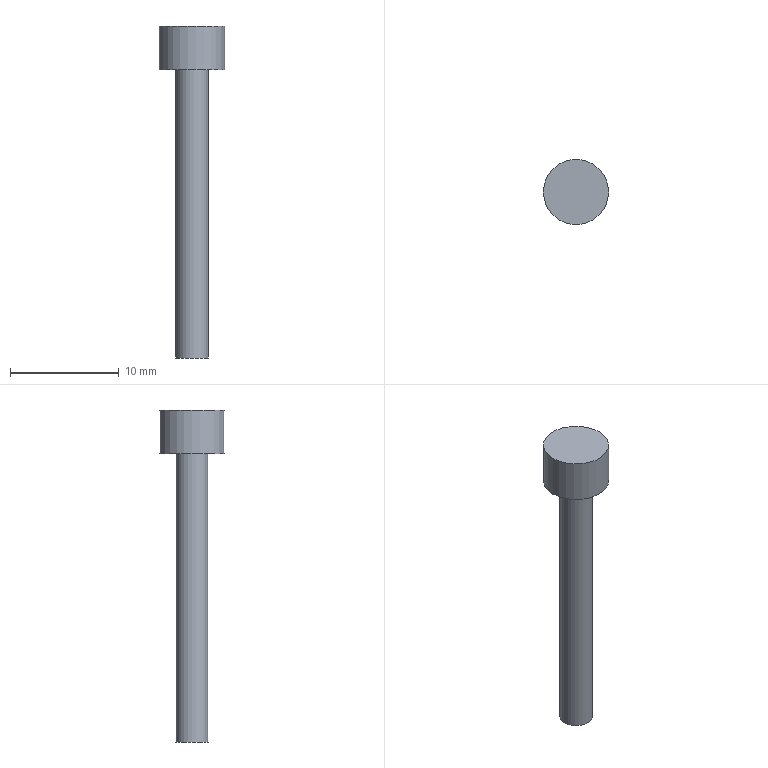Part | STEP file | 1 solid | 5 faces | box 6 x 6 x 30.5 mm | volume 300.415 mm3 | plane 3 | cylinder 2 | commonest cylinder face diameters 3 x1 6 x1
STEP:
#1=CARTESIAN_POINT('',(0.,0.,0.));
#2=DIRECTION('',(0.,0.,1.));
#3=DIRECTION('',(1.,0.,0.));
#4=AXIS2_PLACEMENT_3D('',#1,#2,#3);
#5=CARTESIAN_POINT('',(1371.362,477.495,17.579));
#6=VERTEX_POINT('',#5);
#7=CARTESIAN_POINT('',(1372.862,477.495,17.579));
#8=DIRECTION('',(0.,0.,1.));
#9=DIRECTION('',(-1.,0.,0.));
#10=AXIS2_PLACEMENT_3D('',#7,#8,#9);
#11=CIRCLE('',#10,1.5);
#12=CARTESIAN_POINT('',(1372.862,477.495,17.579));
#13=DIRECTION('',(0.,0.,-1.));
#14=DIRECTION('',(-1.,0.,0.));
#15=AXIS2_PLACEMENT_3D('',#12,#13,#14);
#16=PLANE('',#15);
#17=CARTESIAN_POINT('',(1.5,0.));
#18=CARTESIAN_POINT('',(1.5,-2.598));
#19=CARTESIAN_POINT('',(-0.75,-1.299));
#20=CARTESIAN_POINT('',(-3.,0.));
#21=CARTESIAN_POINT('',(-0.75,1.299));
#22=CARTESIAN_POINT('',(1.5,2.598));
#23=CARTESIAN_POINT('',(1.5,0.));
#24=(BOUNDED_CURVE()B_SPLINE_CURVE(2,(#17,#18,#19,#20,#21,#22,#23),.UNSPECIFIED.,.T.,.F.)B_SPLINE_CURVE_WITH_KNOTS((1,2,2,2,2,1),(-2.094,0.,2.094,4.189,6.283,8.378),.UNSPECIFIED.)CURVE()GEOMETRIC_REPRESENTATION_ITEM()RATIONAL_B_SPLINE_CURVE((1.,0.5,1.,0.5,1.,0.5,1.))REPRESENTATION_ITEM(''));
#25=(GEOMETRIC_REPRESENTATION_CONTEXT(2)PARAMETRIC_REPRESENTATION_CONTEXT()REPRESENTATION_CONTEXT('',''));
#26=DEFINITIONAL_REPRESENTATION('',(#24),#25);
#27=PCURVE('',#16,#26);
#28=CARTESIAN_POINT('',(1372.862,477.495,43.879));
#29=DIRECTION('',(0.,0.,-1.));
#30=DIRECTION('',(-1.,0.,0.));
#31=AXIS2_PLACEMENT_3D('',#28,#29,#30);
#32=CYLINDRICAL_SURFACE('',#31,1.5);
#33=CARTESIAN_POINT('',(6.283,26.3));
#34=DIRECTION('',(-1.,0.));
#35=VECTOR('',#34,1.);
#36=LINE('',#33,#35);
#37=(GEOMETRIC_REPRESENTATION_CONTEXT(2)PARAMETRIC_REPRESENTATION_CONTEXT()REPRESENTATION_CONTEXT('',''));
#38=DEFINITIONAL_REPRESENTATION('',(#36),#37);
#39=PCURVE('',#32,#38);
#40=SURFACE_CURVE('',#11,(#27,#39),.PCURVE_S1.);
#41=EDGE_CURVE('',#6,#6,#40,.T.);
#42=ORIENTED_EDGE('',*,*,#41,.F.);
#43=EDGE_LOOP('',(#42));
#44=FACE_BOUND('',#43,.T.);
#45=ADVANCED_FACE('',(#44),#16,.T.);
#46=ORIENTED_EDGE('',*,*,#41,.T.);
#47=CARTESIAN_POINT('',(1371.362,477.495,44.079));
#48=VERTEX_POINT('',#47);
#49=CARTESIAN_POINT('',(1371.362,477.495,44.079));
#50=CARTESIAN_POINT('',(1371.362,477.495,17.579));
#51=B_SPLINE_CURVE_WITH_KNOTS('',1,(#49,#50),.UNSPECIFIED.,.F.,.F.,(2,2),(-0.2,26.3),.PIECEWISE_BEZIER_KNOTS.);
#52=CARTESIAN_POINT('',(0.,0.));
#53=DIRECTION('',(0.,1.));
#54=VECTOR('',#53,1.);
#55=LINE('',#52,#54);
#56=(GEOMETRIC_REPRESENTATION_CONTEXT(2)PARAMETRIC_REPRESENTATION_CONTEXT()REPRESENTATION_CONTEXT('',''));
#57=DEFINITIONAL_REPRESENTATION('',(#55),#56);
#58=PCURVE('',#32,#57);
#59=CARTESIAN_POINT('',(6.283,0.));
#60=DIRECTION('',(0.,1.));
#61=VECTOR('',#60,1.);
#62=LINE('',#59,#61);
#63=(GEOMETRIC_REPRESENTATION_CONTEXT(2)PARAMETRIC_REPRESENTATION_CONTEXT()REPRESENTATION_CONTEXT('',''));
#64=DEFINITIONAL_REPRESENTATION('',(#62),#63);
#65=PCURVE('',#32,#64);
#66=SEAM_CURVE('',#51,(#58,#65),.PCURVE_S1.);
#67=EDGE_CURVE('',#48,#6,#66,.T.);
#68=ORIENTED_EDGE('',*,*,#67,.F.);
#69=CARTESIAN_POINT('',(1374.362,477.495,44.079));
#70=VERTEX_POINT('',#69);
#71=CARTESIAN_POINT('',(1372.862,477.495,44.079));
#72=DIRECTION('',(0.,0.,1.));
#73=DIRECTION('',(1.,0.,0.));
#74=AXIS2_PLACEMENT_3D('',#71,#72,#73);
#75=CIRCLE('',#74,1.5);
#76=CARTESIAN_POINT('',(3.142,-0.2));
#77=DIRECTION('',(-1.,0.));
#78=VECTOR('',#77,1.);
#79=LINE('',#76,#78);
#80=(GEOMETRIC_REPRESENTATION_CONTEXT(2)PARAMETRIC_REPRESENTATION_CONTEXT()REPRESENTATION_CONTEXT('',''));
#81=DEFINITIONAL_REPRESENTATION('',(#79),#80);
#82=PCURVE('',#32,#81);
#83=CARTESIAN_POINT('',(1372.862,477.495,44.079));
#84=DIRECTION('',(0.,0.,-1.));
#85=DIRECTION('',(-1.,0.,0.));
#86=AXIS2_PLACEMENT_3D('',#83,#84,#85);
#87=PLANE('',#86);
#88=CARTESIAN_POINT('',(-1.5,0.));
#89=CARTESIAN_POINT('',(-1.5,2.598));
#90=CARTESIAN_POINT('',(0.75,1.299));
#91=CARTESIAN_POINT('',(3.,0.));
#92=CARTESIAN_POINT('',(0.75,-1.299));
#93=CARTESIAN_POINT('',(-1.5,-2.598));
#94=CARTESIAN_POINT('',(-1.5,0.));
#95=(BOUNDED_CURVE()B_SPLINE_CURVE(2,(#88,#89,#90,#91,#92,#93,#94),.UNSPECIFIED.,.T.,.F.)B_SPLINE_CURVE_WITH_KNOTS((1,2,2,2,2,1),(-2.094,0.,2.094,4.189,6.283,8.378),.UNSPECIFIED.)CURVE()GEOMETRIC_REPRESENTATION_ITEM()RATIONAL_B_SPLINE_CURVE((1.,0.5,1.,0.5,1.,0.5,1.))REPRESENTATION_ITEM(''));
#96=(GEOMETRIC_REPRESENTATION_CONTEXT(2)PARAMETRIC_REPRESENTATION_CONTEXT()REPRESENTATION_CONTEXT('',''));
#97=DEFINITIONAL_REPRESENTATION('',(#95),#96);
#98=PCURVE('',#87,#97);
#99=SURFACE_CURVE('',#75,(#82,#98),.PCURVE_S1.);
#100=EDGE_CURVE('',#70,#48,#99,.T.);
#101=ORIENTED_EDGE('',*,*,#100,.F.);
#102=CARTESIAN_POINT('',(1372.862,477.495,44.079));
#103=DIRECTION('',(0.,0.,1.));
#104=DIRECTION('',(1.,0.,0.));
#105=AXIS2_PLACEMENT_3D('',#102,#103,#104);
#106=CIRCLE('',#105,1.5);
#107=CARTESIAN_POINT('',(9.425,-0.2));
#108=DIRECTION('',(-1.,0.));
#109=VECTOR('',#108,1.);
#110=LINE('',#107,#109);
#111=(GEOMETRIC_REPRESENTATION_CONTEXT(2)PARAMETRIC_REPRESENTATION_CONTEXT()REPRESENTATION_CONTEXT('',''));
#112=DEFINITIONAL_REPRESENTATION('',(#110),#111);
#113=PCURVE('',#32,#112);
#114=CARTESIAN_POINT('',(-1.5,0.));
#115=CARTESIAN_POINT('',(-1.5,2.598));
#116=CARTESIAN_POINT('',(0.75,1.299));
#117=CARTESIAN_POINT('',(3.,0.));
#118=CARTESIAN_POINT('',(0.75,-1.299));
#119=CARTESIAN_POINT('',(-1.5,-2.598));
#120=CARTESIAN_POINT('',(-1.5,0.));
#121=(BOUNDED_CURVE()B_SPLINE_CURVE(2,(#114,#115,#116,#117,#118,#119,#120),.UNSPECIFIED.,.T.,.F.)B_SPLINE_CURVE_WITH_KNOTS((1,2,2,2,2,1),(-2.094,0.,2.094,4.189,6.283,8.378),.UNSPECIFIED.)CURVE()GEOMETRIC_REPRESENTATION_ITEM()RATIONAL_B_SPLINE_CURVE((1.,0.5,1.,0.5,1.,0.5,1.))REPRESENTATION_ITEM(''));
#122=(GEOMETRIC_REPRESENTATION_CONTEXT(2)PARAMETRIC_REPRESENTATION_CONTEXT()REPRESENTATION_CONTEXT('',''));
#123=DEFINITIONAL_REPRESENTATION('',(#121),#122);
#124=PCURVE('',#87,#123);
#125=SURFACE_CURVE('',#106,(#113,#124),.PCURVE_S1.);
#126=EDGE_CURVE('',#48,#70,#125,.T.);
#127=ORIENTED_EDGE('',*,*,#126,.F.);
#128=ORIENTED_EDGE('',*,*,#67,.T.);
#129=EDGE_LOOP('',(#46,#68,#101,#127,#128));
#130=FACE_BOUND('',#129,.T.);
#131=ADVANCED_FACE('',(#130),#32,.T.);
#132=CARTESIAN_POINT('',(1369.862,477.495,48.079));
#133=VERTEX_POINT('',#132);
#134=CARTESIAN_POINT('',(1372.862,477.495,48.079));
#135=DIRECTION('',(0.,0.,-1.));
#136=DIRECTION('',(-1.,0.,0.));
#137=AXIS2_PLACEMENT_3D('',#134,#135,#136);
#138=CIRCLE('',#137,3.);
#139=CARTESIAN_POINT('',(1372.862,477.495,48.079));
#140=DIRECTION('',(0.,0.,1.));
#141=DIRECTION('',(1.,0.,0.));
#142=AXIS2_PLACEMENT_3D('',#139,#140,#141);
#143=PLANE('',#142);
#144=CARTESIAN_POINT('',(-3.,0.));
#145=CARTESIAN_POINT('',(-3.,5.196));
#146=CARTESIAN_POINT('',(1.5,2.598));
#147=CARTESIAN_POINT('',(6.,0.));
#148=CARTESIAN_POINT('',(1.5,-2.598));
#149=CARTESIAN_POINT('',(-3.,-5.196));
#150=CARTESIAN_POINT('',(-3.,0.));
#151=(BOUNDED_CURVE()B_SPLINE_CURVE(2,(#144,#145,#146,#147,#148,#149,#150),.UNSPECIFIED.,.T.,.F.)B_SPLINE_CURVE_WITH_KNOTS((1,2,2,2,2,1),(-2.094,0.,2.094,4.189,6.283,8.378),.UNSPECIFIED.)CURVE()GEOMETRIC_REPRESENTATION_ITEM()RATIONAL_B_SPLINE_CURVE((1.,0.5,1.,0.5,1.,0.5,1.))REPRESENTATION_ITEM(''));
#152=(GEOMETRIC_REPRESENTATION_CONTEXT(2)PARAMETRIC_REPRESENTATION_CONTEXT()REPRESENTATION_CONTEXT('',''));
#153=DEFINITIONAL_REPRESENTATION('',(#151),#152);
#154=PCURVE('',#143,#153);
#155=CARTESIAN_POINT('',(1372.862,477.495,44.079));
#156=DIRECTION('',(0.,0.,1.));
#157=DIRECTION('',(-1.,0.,0.));
#158=AXIS2_PLACEMENT_3D('',#155,#156,#157);
#159=CYLINDRICAL_SURFACE('',#158,3.);
#160=CARTESIAN_POINT('',(6.283,4.));
#161=DIRECTION('',(-1.,0.));
#162=VECTOR('',#161,1.);
#163=LINE('',#160,#162);
#164=(GEOMETRIC_REPRESENTATION_CONTEXT(2)PARAMETRIC_REPRESENTATION_CONTEXT()REPRESENTATION_CONTEXT('',''));
#165=DEFINITIONAL_REPRESENTATION('',(#163),#164);
#166=PCURVE('',#159,#165);
#167=SURFACE_CURVE('',#138,(#154,#166),.PCURVE_S1.);
#168=EDGE_CURVE('',#133,#133,#167,.T.);
#169=ORIENTED_EDGE('',*,*,#168,.F.);
#170=EDGE_LOOP('',(#169));
#171=FACE_BOUND('',#170,.T.);
#172=ADVANCED_FACE('',(#171),#143,.T.);
#173=ORIENTED_EDGE('',*,*,#100,.T.);
#174=ORIENTED_EDGE('',*,*,#126,.T.);
#175=EDGE_LOOP('',(#173,#174));
#176=FACE_BOUND('',#175,.T.);
#177=CARTESIAN_POINT('',(1375.862,477.495,44.079));
#178=VERTEX_POINT('',#177);
#179=CARTESIAN_POINT('',(1369.862,477.495,44.079));
#180=VERTEX_POINT('',#179);
#181=CARTESIAN_POINT('',(1372.862,477.495,44.079));
#182=DIRECTION('',(0.,0.,1.));
#183=DIRECTION('',(1.,0.,0.));
#184=AXIS2_PLACEMENT_3D('',#181,#182,#183);
#185=CIRCLE('',#184,3.);
#186=CARTESIAN_POINT('',(-3.,0.));
#187=CARTESIAN_POINT('',(-3.,5.196));
#188=CARTESIAN_POINT('',(1.5,2.598));
#189=CARTESIAN_POINT('',(6.,0.));
#190=CARTESIAN_POINT('',(1.5,-2.598));
#191=CARTESIAN_POINT('',(-3.,-5.196));
#192=CARTESIAN_POINT('',(-3.,0.));
#193=(BOUNDED_CURVE()B_SPLINE_CURVE(2,(#186,#187,#188,#189,#190,#191,#192),.UNSPECIFIED.,.T.,.F.)B_SPLINE_CURVE_WITH_KNOTS((1,2,2,2,2,1),(-2.094,0.,2.094,4.189,6.283,8.378),.UNSPECIFIED.)CURVE()GEOMETRIC_REPRESENTATION_ITEM()RATIONAL_B_SPLINE_CURVE((1.,0.5,1.,0.5,1.,0.5,1.))REPRESENTATION_ITEM(''));
#194=(GEOMETRIC_REPRESENTATION_CONTEXT(2)PARAMETRIC_REPRESENTATION_CONTEXT()REPRESENTATION_CONTEXT('',''));
#195=DEFINITIONAL_REPRESENTATION('',(#193),#194);
#196=PCURVE('',#87,#195);
#197=CARTESIAN_POINT('',(3.142,0.));
#198=DIRECTION('',(1.,0.));
#199=VECTOR('',#198,1.);
#200=LINE('',#197,#199);
#201=(GEOMETRIC_REPRESENTATION_CONTEXT(2)PARAMETRIC_REPRESENTATION_CONTEXT()REPRESENTATION_CONTEXT('',''));
#202=DEFINITIONAL_REPRESENTATION('',(#200),#201);
#203=PCURVE('',#159,#202);
#204=SURFACE_CURVE('',#185,(#196,#203),.PCURVE_S1.);
#205=EDGE_CURVE('',#178,#180,#204,.T.);
#206=ORIENTED_EDGE('',*,*,#205,.F.);
#207=CARTESIAN_POINT('',(1372.862,477.495,44.079));
#208=DIRECTION('',(0.,0.,1.));
#209=DIRECTION('',(1.,0.,0.));
#210=AXIS2_PLACEMENT_3D('',#207,#208,#209);
#211=CIRCLE('',#210,3.);
#212=CARTESIAN_POINT('',(-3.,0.));
#213=CARTESIAN_POINT('',(-3.,5.196));
#214=CARTESIAN_POINT('',(1.5,2.598));
#215=CARTESIAN_POINT('',(6.,0.));
#216=CARTESIAN_POINT('',(1.5,-2.598));
#217=CARTESIAN_POINT('',(-3.,-5.196));
#218=CARTESIAN_POINT('',(-3.,0.));
#219=(BOUNDED_CURVE()B_SPLINE_CURVE(2,(#212,#213,#214,#215,#216,#217,#218),.UNSPECIFIED.,.T.,.F.)B_SPLINE_CURVE_WITH_KNOTS((1,2,2,2,2,1),(-2.094,0.,2.094,4.189,6.283,8.378),.UNSPECIFIED.)CURVE()GEOMETRIC_REPRESENTATION_ITEM()RATIONAL_B_SPLINE_CURVE((1.,0.5,1.,0.5,1.,0.5,1.))REPRESENTATION_ITEM(''));
#220=(GEOMETRIC_REPRESENTATION_CONTEXT(2)PARAMETRIC_REPRESENTATION_CONTEXT()REPRESENTATION_CONTEXT('',''));
#221=DEFINITIONAL_REPRESENTATION('',(#219),#220);
#222=PCURVE('',#87,#221);
#223=CARTESIAN_POINT('',(-3.142,0.));
#224=DIRECTION('',(1.,0.));
#225=VECTOR('',#224,1.);
#226=LINE('',#223,#225);
#227=(GEOMETRIC_REPRESENTATION_CONTEXT(2)PARAMETRIC_REPRESENTATION_CONTEXT()REPRESENTATION_CONTEXT('',''));
#228=DEFINITIONAL_REPRESENTATION('',(#226),#227);
#229=PCURVE('',#159,#228);
#230=SURFACE_CURVE('',#211,(#222,#229),.PCURVE_S1.);
#231=EDGE_CURVE('',#180,#178,#230,.T.);
#232=ORIENTED_EDGE('',*,*,#231,.F.);
#233=EDGE_LOOP('',(#206,#232));
#234=FACE_BOUND('',#233,.T.);
#235=ADVANCED_FACE('',(#176,#234),#87,.T.);
#236=ORIENTED_EDGE('',*,*,#168,.T.);
#237=CARTESIAN_POINT('',(1369.862,477.495,44.079));
#238=CARTESIAN_POINT('',(1369.862,477.495,48.079));
#239=B_SPLINE_CURVE_WITH_KNOTS('',1,(#237,#238),.UNSPECIFIED.,.F.,.F.,(2,2),(0.,4.),.PIECEWISE_BEZIER_KNOTS.);
#240=CARTESIAN_POINT('',(0.,0.));
#241=DIRECTION('',(0.,1.));
#242=VECTOR('',#241,1.);
#243=LINE('',#240,#242);
#244=(GEOMETRIC_REPRESENTATION_CONTEXT(2)PARAMETRIC_REPRESENTATION_CONTEXT()REPRESENTATION_CONTEXT('',''));
#245=DEFINITIONAL_REPRESENTATION('',(#243),#244);
#246=PCURVE('',#159,#245);
#247=CARTESIAN_POINT('',(6.283,0.));
#248=DIRECTION('',(0.,1.));
#249=VECTOR('',#248,1.);
#250=LINE('',#247,#249);
#251=(GEOMETRIC_REPRESENTATION_CONTEXT(2)PARAMETRIC_REPRESENTATION_CONTEXT()REPRESENTATION_CONTEXT('',''));
#252=DEFINITIONAL_REPRESENTATION('',(#250),#251);
#253=PCURVE('',#159,#252);
#254=SEAM_CURVE('',#239,(#246,#253),.PCURVE_S1.);
#255=EDGE_CURVE('',#180,#133,#254,.T.);
#256=ORIENTED_EDGE('',*,*,#255,.F.);
#257=ORIENTED_EDGE('',*,*,#231,.T.);
#258=ORIENTED_EDGE('',*,*,#205,.T.);
#259=ORIENTED_EDGE('',*,*,#255,.T.);
#260=EDGE_LOOP('',(#236,#256,#257,#258,#259));
#261=FACE_BOUND('',#260,.T.);
#262=ADVANCED_FACE('',(#261),#159,.T.);
#263=CLOSED_SHELL('',(#45,#131,#172,#235,#262));
#264=MANIFOLD_SOLID_BREP('',#263);
#265=(LENGTH_UNIT()NAMED_UNIT(*)SI_UNIT(.MILLI.,.METRE.));
#266=UNCERTAINTY_MEASURE_WITH_UNIT(LENGTH_MEASURE(0.000005),#265,'','');
#267=(NAMED_UNIT(*)PLANE_ANGLE_UNIT()SI_UNIT($,.RADIAN.));
#268=(NAMED_UNIT(*)SI_UNIT($,.STERADIAN.)SOLID_ANGLE_UNIT());
#269=(GEOMETRIC_REPRESENTATION_CONTEXT(3)GLOBAL_UNCERTAINTY_ASSIGNED_CONTEXT((#266))GLOBAL_UNIT_ASSIGNED_CONTEXT((#265,#267,#268))REPRESENTATION_CONTEXT('',''));
#270=ADVANCED_BREP_SHAPE_REPRESENTATION('',(#4,#264),#269);